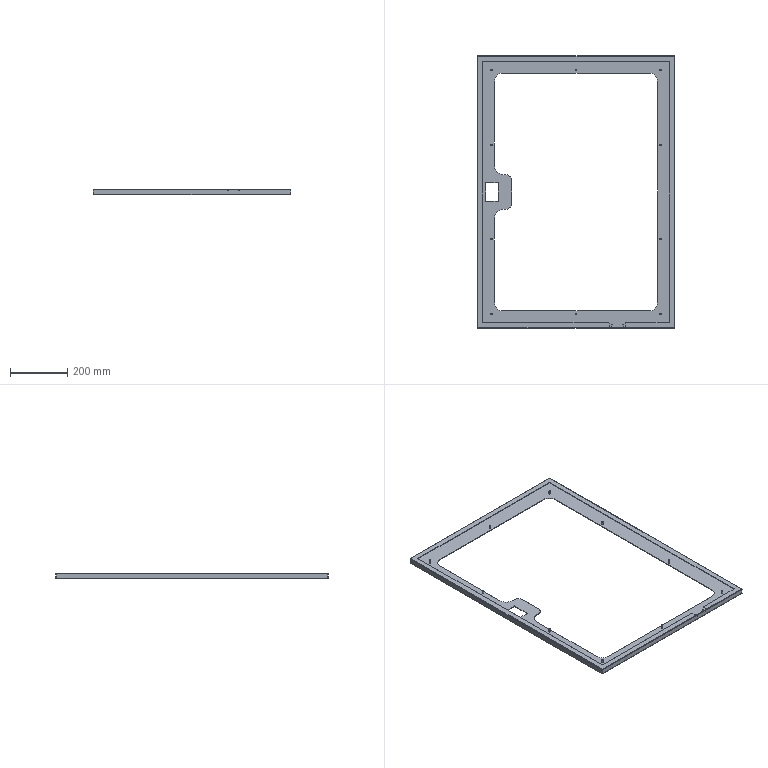Part | STEP file | 11-FG-JX01211 | 1 solid | 103 faces | box 688 x 948 x 20 mm | volume 601333 mm3 | cylinder 50 | plane 45 | sphere 8 | commonest cylinder face diameters 5 x20 4 x12 60 x6 2.5 x4 3 x4 10 x2